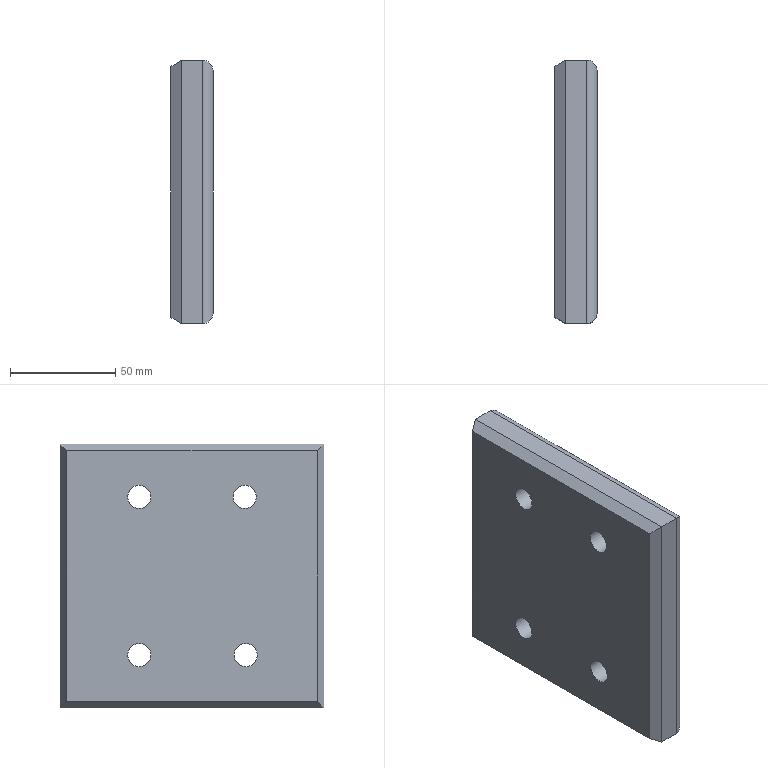Part | NX | features solid 2 | 1 solid | 30 faces | box 20 x 125 x 125 mm | volume 291132 mm3 | plane 14 | cylinder 12 | torus 4 | commonest cylinder face diameters 10 x4 11 x4 17.5 x4
STEP:
#1=CARTESIAN_POINT('',(1235.,-267.5,130.));
#2=VERTEX_POINT('',#1);
#3=CARTESIAN_POINT('',(1225.,-267.5,130.));
#4=VERTEX_POINT('',#3);
#5=CARTESIAN_POINT('',(1240.,-267.5,130.));
#6=DIRECTION('',(-1.,0.,0.));
#7=VECTOR('',#6,1000.);
#8=LINE('',#5,#7);
#9=EDGE_CURVE('',#2,#4,#8,.T.);
#10=ORIENTED_EDGE('',*,*,#9,.F.);
#11=CARTESIAN_POINT('',(1235.,-392.5,130.));
#12=VERTEX_POINT('',#11);
#13=CARTESIAN_POINT('',(1235.,-392.5,130.));
#14=DIRECTION('',(0.,-1.,0.));
#15=VECTOR('',#14,1000.);
#16=LINE('',#13,#15);
#17=EDGE_CURVE('',#12,#2,#16,.F.);
#18=ORIENTED_EDGE('',*,*,#17,.F.);
#19=CARTESIAN_POINT('',(1225.,-392.5,130.));
#20=VERTEX_POINT('',#19);
#21=CARTESIAN_POINT('',(1225.,-392.5,130.));
#22=CARTESIAN_POINT('',(1228.333,-392.5,130.));
#23=CARTESIAN_POINT('',(1231.667,-392.5,130.));
#24=CARTESIAN_POINT('',(1235.,-392.5,130.));
#25=B_SPLINE_CURVE_WITH_KNOTS('',3,(#21,#22,#23,#24),.UNSPECIFIED.,.F.,.F.,(4,4),(0.25,0.75),.UNSPECIFIED.);
#26=EDGE_CURVE('',#12,#20,#25,.F.);
#27=ORIENTED_EDGE('',*,*,#26,.T.);
#28=CARTESIAN_POINT('',(1225.,-392.5,130.));
#29=DIRECTION('',(0.,-1.,0.));
#30=VECTOR('',#29,1000.);
#31=LINE('',#28,#30);
#32=EDGE_CURVE('',#4,#20,#31,.T.);
#33=ORIENTED_EDGE('',*,*,#32,.F.);
#34=EDGE_LOOP('',(#10,#18,#27,#33));
#35=FACE_BOUND('',#34,.T.);
#36=CARTESIAN_POINT('',(1240.,-392.5,130.));
#37=DIRECTION('',(0.,0.,-1.));
#38=DIRECTION('',(1.,0.,0.));
#39=AXIS2_PLACEMENT_3D('',#36,#37,#38);
#40=PLANE('',#39);
#41=ADVANCED_FACE('',(#35),#40,.T.);
#42=ORIENTED_EDGE('',*,*,#26,.F.);
#43=CARTESIAN_POINT('',(1235.,-392.5,255.));
#44=VERTEX_POINT('',#43);
#45=CARTESIAN_POINT('',(1235.,-392.5,200.));
#46=DIRECTION('',(0.,0.,1.));
#47=VECTOR('',#46,1000.);
#48=LINE('',#45,#47);
#49=EDGE_CURVE('',#44,#12,#48,.F.);
#50=ORIENTED_EDGE('',*,*,#49,.F.);
#51=CARTESIAN_POINT('',(1225.,-392.5,255.));
#52=VERTEX_POINT('',#51);
#53=CARTESIAN_POINT('',(1240.,-392.5,255.));
#54=DIRECTION('',(-1.,0.,0.));
#55=VECTOR('',#54,1000.);
#56=LINE('',#53,#55);
#57=EDGE_CURVE('',#44,#52,#56,.T.);
#58=ORIENTED_EDGE('',*,*,#57,.T.);
#59=CARTESIAN_POINT('',(1225.,-392.5,255.));
#60=DIRECTION('',(0.,0.,1.));
#61=VECTOR('',#60,1000.);
#62=LINE('',#59,#61);
#63=EDGE_CURVE('',#20,#52,#62,.T.);
#64=ORIENTED_EDGE('',*,*,#63,.F.);
#65=EDGE_LOOP('',(#42,#50,#58,#64));
#66=FACE_BOUND('',#65,.T.);
#67=CARTESIAN_POINT('',(1240.,-392.5,200.));
#68=DIRECTION('',(0.,-1.,0.));
#69=DIRECTION('',(0.,0.,-1.));
#70=AXIS2_PLACEMENT_3D('',#67,#68,#69);
#71=PLANE('',#70);
#72=ADVANCED_FACE('',(#66),#71,.T.);
#73=ORIENTED_EDGE('',*,*,#57,.F.);
#74=CARTESIAN_POINT('',(1235.,-267.5,255.));
#75=VERTEX_POINT('',#74);
#76=CARTESIAN_POINT('',(1235.,-392.5,255.));
#77=DIRECTION('',(0.,-1.,0.));
#78=VECTOR('',#77,1000.);
#79=LINE('',#76,#78);
#80=EDGE_CURVE('',#75,#44,#79,.T.);
#81=ORIENTED_EDGE('',*,*,#80,.F.);
#82=CARTESIAN_POINT('',(1225.,-267.5,255.));
#83=VERTEX_POINT('',#82);
#84=CARTESIAN_POINT('',(1240.,-267.5,255.));
#85=DIRECTION('',(-1.,0.,0.));
#86=VECTOR('',#85,1000.);
#87=LINE('',#84,#86);
#88=EDGE_CURVE('',#75,#83,#87,.T.);
#89=ORIENTED_EDGE('',*,*,#88,.T.);
#90=CARTESIAN_POINT('',(1225.,-392.5,255.));
#91=DIRECTION('',(0.,1.,0.));
#92=VECTOR('',#91,1000.);
#93=LINE('',#90,#92);
#94=EDGE_CURVE('',#52,#83,#93,.T.);
#95=ORIENTED_EDGE('',*,*,#94,.F.);
#96=EDGE_LOOP('',(#73,#81,#89,#95));
#97=FACE_BOUND('',#96,.T.);
#98=CARTESIAN_POINT('',(1240.,-392.5,255.));
#99=DIRECTION('',(0.,0.,-1.));
#100=DIRECTION('',(1.,0.,0.));
#101=AXIS2_PLACEMENT_3D('',#98,#99,#100);
#102=PLANE('',#101);
#103=ADVANCED_FACE('',(#97),#102,.F.);
#104=ORIENTED_EDGE('',*,*,#88,.F.);
#105=CARTESIAN_POINT('',(1235.,-267.5,255.));
#106=DIRECTION('',(0.,0.,1.));
#107=VECTOR('',#106,1000.);
#108=LINE('',#105,#107);
#109=EDGE_CURVE('',#2,#75,#108,.T.);
#110=ORIENTED_EDGE('',*,*,#109,.F.);
#111=ORIENTED_EDGE('',*,*,#9,.T.);
#112=CARTESIAN_POINT('',(1225.,-267.5,200.));
#113=DIRECTION('',(0.,0.,-1.));
#114=VECTOR('',#113,1000.);
#115=LINE('',#112,#114);
#116=EDGE_CURVE('',#83,#4,#115,.T.);
#117=ORIENTED_EDGE('',*,*,#116,.F.);
#118=EDGE_LOOP('',(#104,#110,#111,#117));
#119=FACE_BOUND('',#118,.T.);
#120=CARTESIAN_POINT('',(1240.,-267.5,200.));
#121=DIRECTION('',(0.,-1.,0.));
#122=DIRECTION('',(0.,0.,-1.));
#123=AXIS2_PLACEMENT_3D('',#120,#121,#122);
#124=PLANE('',#123);
#125=ADVANCED_FACE('',(#119),#124,.F.);
#126=CARTESIAN_POINT('',(1240.,-355.,218.25));
#127=VERTEX_POINT('',#126);
#128=CARTESIAN_POINT('',(1240.,-355.,230.));
#129=DIRECTION('',(1.,0.,0.));
#130=DIRECTION('',(0.,0.,-1.));
#131=AXIS2_PLACEMENT_3D('',#128,#129,#130);
#132=CIRCLE('',#131,11.75);
#133=EDGE_CURVE('',#127,#127,#132,.T.);
#134=ORIENTED_EDGE('',*,*,#133,.F.);
#135=EDGE_LOOP('',(#134));
#136=FACE_BOUND('',#135,.T.);
#137=CARTESIAN_POINT('',(1240.,-305.,218.25));
#138=VERTEX_POINT('',#137);
#139=CARTESIAN_POINT('',(1240.,-305.,230.));
#140=DIRECTION('',(1.,0.,0.));
#141=DIRECTION('',(0.,0.,-1.));
#142=AXIS2_PLACEMENT_3D('',#139,#140,#141);
#143=CIRCLE('',#142,11.75);
#144=EDGE_CURVE('',#138,#138,#143,.T.);
#145=ORIENTED_EDGE('',*,*,#144,.F.);
#146=EDGE_LOOP('',(#145));
#147=FACE_BOUND('',#146,.T.);
#148=CARTESIAN_POINT('',(1240.,-305.,143.25));
#149=VERTEX_POINT('',#148);
#150=CARTESIAN_POINT('',(1240.,-305.,155.));
#151=DIRECTION('',(1.,0.,0.));
#152=DIRECTION('',(0.,0.,-1.));
#153=AXIS2_PLACEMENT_3D('',#150,#151,#152);
#154=CIRCLE('',#153,11.75);
#155=EDGE_CURVE('',#149,#149,#154,.T.);
#156=ORIENTED_EDGE('',*,*,#155,.F.);
#157=EDGE_LOOP('',(#156));
#158=FACE_BOUND('',#157,.T.);
#159=CARTESIAN_POINT('',(1240.,-355.5,143.25));
#160=VERTEX_POINT('',#159);
#161=CARTESIAN_POINT('',(1240.,-355.5,155.));
#162=DIRECTION('',(1.,0.,0.));
#163=DIRECTION('',(0.,0.,-1.));
#164=AXIS2_PLACEMENT_3D('',#161,#162,#163);
#165=CIRCLE('',#164,11.75);
#166=EDGE_CURVE('',#160,#160,#165,.T.);
#167=ORIENTED_EDGE('',*,*,#166,.F.);
#168=EDGE_LOOP('',(#167));
#169=FACE_BOUND('',#168,.T.);
#170=CARTESIAN_POINT('',(1240.,-387.5,135.));
#171=VERTEX_POINT('',#170);
#172=CARTESIAN_POINT('',(1240.,-387.5,250.));
#173=VERTEX_POINT('',#172);
#174=CARTESIAN_POINT('',(1240.,-387.5,200.));
#175=DIRECTION('',(0.,0.,-1.));
#176=VECTOR('',#175,1000.);
#177=LINE('',#174,#176);
#178=EDGE_CURVE('',#171,#173,#177,.F.);
#179=ORIENTED_EDGE('',*,*,#178,.F.);
#180=CARTESIAN_POINT('',(1240.,-272.5,135.));
#181=VERTEX_POINT('',#180);
#182=CARTESIAN_POINT('',(1240.,-392.5,135.));
#183=DIRECTION('',(0.,1.,0.));
#184=VECTOR('',#183,1000.);
#185=LINE('',#182,#184);
#186=EDGE_CURVE('',#181,#171,#185,.F.);
#187=ORIENTED_EDGE('',*,*,#186,.F.);
#188=CARTESIAN_POINT('',(1240.,-272.5,250.));
#189=VERTEX_POINT('',#188);
#190=CARTESIAN_POINT('',(1240.,-272.5,130.));
#191=DIRECTION('',(0.,0.,-1.));
#192=VECTOR('',#191,1000.);
#193=LINE('',#190,#192);
#194=EDGE_CURVE('',#189,#181,#193,.T.);
#195=ORIENTED_EDGE('',*,*,#194,.F.);
#196=CARTESIAN_POINT('',(1240.,-267.5,250.));
#197=DIRECTION('',(0.,1.,0.));
#198=VECTOR('',#197,1000.);
#199=LINE('',#196,#198);
#200=EDGE_CURVE('',#173,#189,#199,.T.);
#201=ORIENTED_EDGE('',*,*,#200,.F.);
#202=EDGE_LOOP('',(#179,#187,#195,#201));
#203=FACE_BOUND('',#202,.T.);
#204=CARTESIAN_POINT('',(1240.,-392.5,200.));
#205=DIRECTION('',(-1.,0.,0.));
#206=DIRECTION('',(0.,0.,-1.));
#207=AXIS2_PLACEMENT_3D('',#204,#205,#206);
#208=PLANE('',#207);
#209=ADVANCED_FACE('',(#136,#147,#158,#169,#203),#208,.F.);
#210=CARTESIAN_POINT('',(1220.,-389.5,133.));
#211=VERTEX_POINT('',#210);
#212=CARTESIAN_POINT('',(1220.,-270.5,133.));
#213=VERTEX_POINT('',#212);
#214=CARTESIAN_POINT('',(1220.,-267.5,133.));
#215=DIRECTION('',(0.,-1.,0.));
#216=VECTOR('',#215,1000.);
#217=LINE('',#214,#216);
#218=EDGE_CURVE('',#211,#213,#217,.F.);
#219=ORIENTED_EDGE('',*,*,#218,.F.);
#220=CARTESIAN_POINT('',(1220.,-389.5,252.));
#221=VERTEX_POINT('',#220);
#222=CARTESIAN_POINT('',(1220.,-389.5,130.));
#223=DIRECTION('',(0.,0.,1.));
#224=VECTOR('',#223,1000.);
#225=LINE('',#222,#224);
#226=EDGE_CURVE('',#221,#211,#225,.F.);
#227=ORIENTED_EDGE('',*,*,#226,.F.);
#228=CARTESIAN_POINT('',(1220.,-270.5,252.));
#229=VERTEX_POINT('',#228);
#230=CARTESIAN_POINT('',(1220.,-392.5,252.));
#231=DIRECTION('',(0.,1.,0.));
#232=VECTOR('',#231,1000.);
#233=LINE('',#230,#232);
#234=EDGE_CURVE('',#229,#221,#233,.F.);
#235=ORIENTED_EDGE('',*,*,#234,.F.);
#236=CARTESIAN_POINT('',(1220.,-270.5,200.));
#237=DIRECTION('',(0.,0.,-1.));
#238=VECTOR('',#237,1000.);
#239=LINE('',#236,#238);
#240=EDGE_CURVE('',#213,#229,#239,.F.);
#241=ORIENTED_EDGE('',*,*,#240,.F.);
#242=EDGE_LOOP('',(#219,#227,#235,#241));
#243=FACE_BOUND('',#242,.T.);
#244=CARTESIAN_POINT('',(1220.,-305.,224.5));
#245=VERTEX_POINT('',#244);
#246=CARTESIAN_POINT('',(1220.,-305.,230.));
#247=DIRECTION('',(1.,0.,0.));
#248=DIRECTION('',(0.,0.,-1.));
#249=AXIS2_PLACEMENT_3D('',#246,#247,#248);
#250=CIRCLE('',#249,5.5);
#251=EDGE_CURVE('',#245,#245,#250,.F.);
#252=ORIENTED_EDGE('',*,*,#251,.F.);
#253=EDGE_LOOP('',(#252));
#254=FACE_BOUND('',#253,.T.);
#255=CARTESIAN_POINT('',(1220.,-355.,224.5));
#256=VERTEX_POINT('',#255);
#257=CARTESIAN_POINT('',(1220.,-355.,230.));
#258=DIRECTION('',(1.,0.,0.));
#259=DIRECTION('',(0.,0.,-1.));
#260=AXIS2_PLACEMENT_3D('',#257,#258,#259);
#261=CIRCLE('',#260,5.5);
#262=EDGE_CURVE('',#256,#256,#261,.F.);
#263=ORIENTED_EDGE('',*,*,#262,.F.);
#264=EDGE_LOOP('',(#263));
#265=FACE_BOUND('',#264,.T.);
#266=CARTESIAN_POINT('',(1220.,-305.,149.5));
#267=VERTEX_POINT('',#266);
#268=CARTESIAN_POINT('',(1220.,-305.,155.));
#269=DIRECTION('',(1.,0.,0.));
#270=DIRECTION('',(0.,0.,-1.));
#271=AXIS2_PLACEMENT_3D('',#268,#269,#270);
#272=CIRCLE('',#271,5.5);
#273=EDGE_CURVE('',#267,#267,#272,.F.);
#274=ORIENTED_EDGE('',*,*,#273,.F.);
#275=EDGE_LOOP('',(#274));
#276=FACE_BOUND('',#275,.T.);
#277=CARTESIAN_POINT('',(1220.,-355.5,149.5));
#278=VERTEX_POINT('',#277);
#279=CARTESIAN_POINT('',(1220.,-355.5,155.));
#280=DIRECTION('',(1.,0.,0.));
#281=DIRECTION('',(0.,0.,-1.));
#282=AXIS2_PLACEMENT_3D('',#279,#280,#281);
#283=CIRCLE('',#282,5.5);
#284=EDGE_CURVE('',#278,#278,#283,.F.);
#285=ORIENTED_EDGE('',*,*,#284,.F.);
#286=EDGE_LOOP('',(#285));
#287=FACE_BOUND('',#286,.T.);
#288=CARTESIAN_POINT('',(1220.,-392.5,200.));
#289=DIRECTION('',(-1.,0.,0.));
#290=DIRECTION('',(0.,0.,-1.));
#291=AXIS2_PLACEMENT_3D('',#288,#289,#290);
#292=PLANE('',#291);
#293=ADVANCED_FACE('',(#243,#254,#265,#276,#287),#292,.T.);
#294=CARTESIAN_POINT('',(1228.,-355.5,149.5));
#295=VERTEX_POINT('',#294);
#296=CARTESIAN_POINT('',(1228.,-355.5,155.));
#297=DIRECTION('',(1.,0.,0.));
#298=DIRECTION('',(0.,0.,-1.));
#299=AXIS2_PLACEMENT_3D('',#296,#297,#298);
#300=CIRCLE('',#299,5.5);
#301=EDGE_CURVE('',#295,#295,#300,.T.);
#302=ORIENTED_EDGE('',*,*,#301,.T.);
#303=EDGE_LOOP('',(#302));
#304=FACE_BOUND('',#303,.T.);
#305=ORIENTED_EDGE('',*,*,#284,.T.);
#306=EDGE_LOOP('',(#305));
#307=FACE_BOUND('',#306,.T.);
#308=CARTESIAN_POINT('',(1190.,-355.5,155.));
#309=DIRECTION('',(-1.,0.,0.));
#310=DIRECTION('',(0.,0.,-1.));
#311=AXIS2_PLACEMENT_3D('',#308,#309,#310);
#312=CYLINDRICAL_SURFACE('',#311,5.5);
#313=ADVANCED_FACE('',(#304,#307),#312,.F.);
#314=ORIENTED_EDGE('',*,*,#301,.F.);
#315=EDGE_LOOP('',(#314));
#316=FACE_BOUND('',#315,.T.);
#317=CARTESIAN_POINT('',(1228.,-355.5,146.25));
#318=VERTEX_POINT('',#317);
#319=CARTESIAN_POINT('',(1228.,-355.5,155.));
#320=DIRECTION('',(1.,0.,0.));
#321=DIRECTION('',(0.,0.,-1.));
#322=AXIS2_PLACEMENT_3D('',#319,#320,#321);
#323=CIRCLE('',#322,8.75);
#324=EDGE_CURVE('',#318,#318,#323,.T.);
#325=ORIENTED_EDGE('',*,*,#324,.T.);
#326=EDGE_LOOP('',(#325));
#327=FACE_BOUND('',#326,.T.);
#328=CARTESIAN_POINT('',(1228.,-355.5,155.));
#329=DIRECTION('',(-1.,0.,0.));
#330=DIRECTION('',(0.,0.,-1.));
#331=AXIS2_PLACEMENT_3D('',#328,#329,#330);
#332=PLANE('',#331);
#333=ADVANCED_FACE('',(#316,#327),#332,.F.);
#334=CARTESIAN_POINT('',(1237.,-355.5,146.25));
#335=VERTEX_POINT('',#334);
#336=CARTESIAN_POINT('',(1237.,-355.5,155.));
#337=DIRECTION('',(1.,0.,0.));
#338=DIRECTION('',(0.,0.,-1.));
#339=AXIS2_PLACEMENT_3D('',#336,#337,#338);
#340=CIRCLE('',#339,8.75);
#341=EDGE_CURVE('',#335,#335,#340,.F.);
#342=ORIENTED_EDGE('',*,*,#341,.F.);
#343=EDGE_LOOP('',(#342));
#344=FACE_BOUND('',#343,.T.);
#345=ORIENTED_EDGE('',*,*,#324,.F.);
#346=EDGE_LOOP('',(#345));
#347=FACE_BOUND('',#346,.T.);
#348=CARTESIAN_POINT('',(1240.,-355.5,155.));
#349=DIRECTION('',(-1.,0.,0.));
#350=DIRECTION('',(0.,0.,-1.));
#351=AXIS2_PLACEMENT_3D('',#348,#349,#350);
#352=CYLINDRICAL_SURFACE('',#351,8.75);
#353=ADVANCED_FACE('',(#344,#347),#352,.F.);
#354=CARTESIAN_POINT('',(1228.,-305.,149.5));
#355=VERTEX_POINT('',#354);
#356=CARTESIAN_POINT('',(1228.,-305.,155.));
#357=DIRECTION('',(1.,0.,0.));
#358=DIRECTION('',(0.,0.,-1.));
#359=AXIS2_PLACEMENT_3D('',#356,#357,#358);
#360=CIRCLE('',#359,5.5);
#361=EDGE_CURVE('',#355,#355,#360,.T.);
#362=ORIENTED_EDGE('',*,*,#361,.T.);
#363=EDGE_LOOP('',(#362));
#364=FACE_BOUND('',#363,.T.);
#365=ORIENTED_EDGE('',*,*,#273,.T.);
#366=EDGE_LOOP('',(#365));
#367=FACE_BOUND('',#366,.T.);
#368=CARTESIAN_POINT('',(1190.,-305.,155.));
#369=DIRECTION('',(-1.,0.,0.));
#370=DIRECTION('',(0.,0.,-1.));
#371=AXIS2_PLACEMENT_3D('',#368,#369,#370);
#372=CYLINDRICAL_SURFACE('',#371,5.5);
#373=ADVANCED_FACE('',(#364,#367),#372,.F.);
#374=ORIENTED_EDGE('',*,*,#361,.F.);
#375=EDGE_LOOP('',(#374));
#376=FACE_BOUND('',#375,.T.);
#377=CARTESIAN_POINT('',(1228.,-305.,146.25));
#378=VERTEX_POINT('',#377);
#379=CARTESIAN_POINT('',(1228.,-305.,155.));
#380=DIRECTION('',(1.,0.,0.));
#381=DIRECTION('',(0.,0.,-1.));
#382=AXIS2_PLACEMENT_3D('',#379,#380,#381);
#383=CIRCLE('',#382,8.75);
#384=EDGE_CURVE('',#378,#378,#383,.T.);
#385=ORIENTED_EDGE('',*,*,#384,.T.);
#386=EDGE_LOOP('',(#385));
#387=FACE_BOUND('',#386,.T.);
#388=CARTESIAN_POINT('',(1228.,-305.,155.));
#389=DIRECTION('',(-1.,0.,0.));
#390=DIRECTION('',(0.,0.,-1.));
#391=AXIS2_PLACEMENT_3D('',#388,#389,#390);
#392=PLANE('',#391);
#393=ADVANCED_FACE('',(#376,#387),#392,.F.);
#394=CARTESIAN_POINT('',(1237.,-305.,146.25));
#395=VERTEX_POINT('',#394);
#396=CARTESIAN_POINT('',(1237.,-305.,155.));
#397=DIRECTION('',(1.,0.,0.));
#398=DIRECTION('',(0.,0.,-1.));
#399=AXIS2_PLACEMENT_3D('',#396,#397,#398);
#400=CIRCLE('',#399,8.75);
#401=EDGE_CURVE('',#395,#395,#400,.F.);
#402=ORIENTED_EDGE('',*,*,#401,.F.);
#403=EDGE_LOOP('',(#402));
#404=FACE_BOUND('',#403,.T.);
#405=ORIENTED_EDGE('',*,*,#384,.F.);
#406=EDGE_LOOP('',(#405));
#407=FACE_BOUND('',#406,.T.);
#408=CARTESIAN_POINT('',(1240.,-305.,155.));
#409=DIRECTION('',(-1.,0.,0.));
#410=DIRECTION('',(0.,0.,-1.));
#411=AXIS2_PLACEMENT_3D('',#408,#409,#410);
#412=CYLINDRICAL_SURFACE('',#411,8.75);
#413=ADVANCED_FACE('',(#404,#407),#412,.F.);
#414=CARTESIAN_POINT('',(1228.,-355.,224.5));
#415=VERTEX_POINT('',#414);
#416=CARTESIAN_POINT('',(1228.,-355.,230.));
#417=DIRECTION('',(1.,0.,0.));
#418=DIRECTION('',(0.,0.,-1.));
#419=AXIS2_PLACEMENT_3D('',#416,#417,#418);
#420=CIRCLE('',#419,5.5);
#421=EDGE_CURVE('',#415,#415,#420,.T.);
#422=ORIENTED_EDGE('',*,*,#421,.T.);
#423=EDGE_LOOP('',(#422));
#424=FACE_BOUND('',#423,.T.);
#425=ORIENTED_EDGE('',*,*,#262,.T.);
#426=EDGE_LOOP('',(#425));
#427=FACE_BOUND('',#426,.T.);
#428=CARTESIAN_POINT('',(1190.,-355.,230.));
#429=DIRECTION('',(-1.,0.,0.));
#430=DIRECTION('',(0.,0.,-1.));
#431=AXIS2_PLACEMENT_3D('',#428,#429,#430);
#432=CYLINDRICAL_SURFACE('',#431,5.5);
#433=ADVANCED_FACE('',(#424,#427),#432,.F.);
#434=ORIENTED_EDGE('',*,*,#421,.F.);
#435=EDGE_LOOP('',(#434));
#436=FACE_BOUND('',#435,.T.);
#437=CARTESIAN_POINT('',(1228.,-355.,221.25));
#438=VERTEX_POINT('',#437);
#439=CARTESIAN_POINT('',(1228.,-355.,230.));
#440=DIRECTION('',(1.,0.,0.));
#441=DIRECTION('',(0.,0.,-1.));
#442=AXIS2_PLACEMENT_3D('',#439,#440,#441);
#443=CIRCLE('',#442,8.75);
#444=EDGE_CURVE('',#438,#438,#443,.T.);
#445=ORIENTED_EDGE('',*,*,#444,.T.);
#446=EDGE_LOOP('',(#445));
#447=FACE_BOUND('',#446,.T.);
#448=CARTESIAN_POINT('',(1228.,-355.,230.));
#449=DIRECTION('',(-1.,0.,0.));
#450=DIRECTION('',(0.,0.,-1.));
#451=AXIS2_PLACEMENT_3D('',#448,#449,#450);
#452=PLANE('',#451);
#453=ADVANCED_FACE('',(#436,#447),#452,.F.);
#454=CARTESIAN_POINT('',(1237.,-355.,221.25));
#455=VERTEX_POINT('',#454);
#456=CARTESIAN_POINT('',(1237.,-355.,230.));
#457=DIRECTION('',(1.,0.,0.));
#458=DIRECTION('',(0.,0.,-1.));
#459=AXIS2_PLACEMENT_3D('',#456,#457,#458);
#460=CIRCLE('',#459,8.75);
#461=EDGE_CURVE('',#455,#455,#460,.F.);
#462=ORIENTED_EDGE('',*,*,#461,.F.);
#463=EDGE_LOOP('',(#462));
#464=FACE_BOUND('',#463,.T.);
#465=ORIENTED_EDGE('',*,*,#444,.F.);
#466=EDGE_LOOP('',(#465));
#467=FACE_BOUND('',#466,.T.);
#468=CARTESIAN_POINT('',(1240.,-355.,230.));
#469=DIRECTION('',(-1.,0.,0.));
#470=DIRECTION('',(0.,0.,-1.));
#471=AXIS2_PLACEMENT_3D('',#468,#469,#470);
#472=CYLINDRICAL_SURFACE('',#471,8.75);
#473=ADVANCED_FACE('',(#464,#467),#472,.F.);
#474=CARTESIAN_POINT('',(1228.,-305.,224.5));
#475=VERTEX_POINT('',#474);
#476=CARTESIAN_POINT('',(1228.,-305.,230.));
#477=DIRECTION('',(1.,0.,0.));
#478=DIRECTION('',(0.,0.,-1.));
#479=AXIS2_PLACEMENT_3D('',#476,#477,#478);
#480=CIRCLE('',#479,5.5);
#481=EDGE_CURVE('',#475,#475,#480,.T.);
#482=ORIENTED_EDGE('',*,*,#481,.T.);
#483=EDGE_LOOP('',(#482));
#484=FACE_BOUND('',#483,.T.);
#485=ORIENTED_EDGE('',*,*,#251,.T.);
#486=EDGE_LOOP('',(#485));
#487=FACE_BOUND('',#486,.T.);
#488=CARTESIAN_POINT('',(1190.,-305.,230.));
#489=DIRECTION('',(-1.,0.,0.));
#490=DIRECTION('',(0.,0.,-1.));
#491=AXIS2_PLACEMENT_3D('',#488,#489,#490);
#492=CYLINDRICAL_SURFACE('',#491,5.5);
#493=ADVANCED_FACE('',(#484,#487),#492,.F.);
#494=ORIENTED_EDGE('',*,*,#481,.F.);
#495=EDGE_LOOP('',(#494));
#496=FACE_BOUND('',#495,.T.);
#497=CARTESIAN_POINT('',(1228.,-305.,221.25));
#498=VERTEX_POINT('',#497);
#499=CARTESIAN_POINT('',(1228.,-305.,230.));
#500=DIRECTION('',(1.,0.,0.));
#501=DIRECTION('',(0.,0.,-1.));
#502=AXIS2_PLACEMENT_3D('',#499,#500,#501);
#503=CIRCLE('',#502,8.75);
#504=EDGE_CURVE('',#498,#498,#503,.T.);
#505=ORIENTED_EDGE('',*,*,#504,.T.);
#506=EDGE_LOOP('',(#505));
#507=FACE_BOUND('',#506,.T.);
#508=CARTESIAN_POINT('',(1228.,-305.,230.));
#509=DIRECTION('',(-1.,0.,0.));
#510=DIRECTION('',(0.,0.,-1.));
#511=AXIS2_PLACEMENT_3D('',#508,#509,#510);
#512=PLANE('',#511);
#513=ADVANCED_FACE('',(#496,#507),#512,.F.);
#514=CARTESIAN_POINT('',(1237.,-305.,221.25));
#515=VERTEX_POINT('',#514);
#516=CARTESIAN_POINT('',(1237.,-305.,230.));
#517=DIRECTION('',(1.,0.,0.));
#518=DIRECTION('',(0.,0.,-1.));
#519=AXIS2_PLACEMENT_3D('',#516,#517,#518);
#520=CIRCLE('',#519,8.75);
#521=EDGE_CURVE('',#515,#515,#520,.F.);
#522=ORIENTED_EDGE('',*,*,#521,.F.);
#523=EDGE_LOOP('',(#522));
#524=FACE_BOUND('',#523,.T.);
#525=ORIENTED_EDGE('',*,*,#504,.F.);
#526=EDGE_LOOP('',(#525));
#527=FACE_BOUND('',#526,.T.);
#528=CARTESIAN_POINT('',(1240.,-305.,230.));
#529=DIRECTION('',(-1.,0.,0.));
#530=DIRECTION('',(0.,0.,-1.));
#531=AXIS2_PLACEMENT_3D('',#528,#529,#530);
#532=CYLINDRICAL_SURFACE('',#531,8.75);
#533=ADVANCED_FACE('',(#524,#527),#532,.F.);
#534=CARTESIAN_POINT('',(1235.,-272.5,135.));
#535=DIRECTION('',(0.,0.7071,0.7071));
#536=DIRECTION('',(0.,-0.7071,0.7071));
#537=AXIS2_PLACEMENT_3D('',#534,#535,#536);
#538=ELLIPSE('',#537,7.071,5.);
#539=EDGE_CURVE('',#2,#181,#538,.F.);
#540=ORIENTED_EDGE('',*,*,#539,.T.);
#541=ORIENTED_EDGE('',*,*,#186,.T.);
#542=CARTESIAN_POINT('',(1235.,-387.5,135.));
#543=DIRECTION('',(0.,0.7071,-0.7071));
#544=DIRECTION('',(0.,0.7071,0.7071));
#545=AXIS2_PLACEMENT_3D('',#542,#543,#544);
#546=ELLIPSE('',#545,7.071,5.);
#547=EDGE_CURVE('',#171,#12,#546,.T.);
#548=ORIENTED_EDGE('',*,*,#547,.T.);
#549=ORIENTED_EDGE('',*,*,#17,.T.);
#550=EDGE_LOOP('',(#540,#541,#548,#549));
#551=FACE_BOUND('',#550,.T.);
#552=CARTESIAN_POINT('',(1235.,-392.5,135.));
#553=DIRECTION('',(0.,-1.,0.));
#554=DIRECTION('',(0.,0.,-1.));
#555=AXIS2_PLACEMENT_3D('',#552,#553,#554);
#556=CYLINDRICAL_SURFACE('',#555,5.);
#557=ADVANCED_FACE('',(#551),#556,.T.);
#558=ORIENTED_EDGE('',*,*,#547,.F.);
#559=ORIENTED_EDGE('',*,*,#178,.T.);
#560=CARTESIAN_POINT('',(1235.,-387.5,250.));
#561=DIRECTION('',(0.,-0.7071,-0.7071));
#562=DIRECTION('',(0.,-0.7071,0.7071));
#563=AXIS2_PLACEMENT_3D('',#560,#561,#562);
#564=ELLIPSE('',#563,7.071,5.);
#565=EDGE_CURVE('',#173,#44,#564,.T.);
#566=ORIENTED_EDGE('',*,*,#565,.T.);
#567=ORIENTED_EDGE('',*,*,#49,.T.);
#568=EDGE_LOOP('',(#558,#559,#566,#567));
#569=FACE_BOUND('',#568,.T.);
#570=CARTESIAN_POINT('',(1235.,-387.5,200.));
#571=DIRECTION('',(0.,0.,1.));
#572=DIRECTION('',(-1.,0.,0.));
#573=AXIS2_PLACEMENT_3D('',#570,#571,#572);
#574=CYLINDRICAL_SURFACE('',#573,5.);
#575=ADVANCED_FACE('',(#569),#574,.T.);
#576=ORIENTED_EDGE('',*,*,#539,.F.);
#577=ORIENTED_EDGE('',*,*,#109,.T.);
#578=CARTESIAN_POINT('',(1235.,-272.5,250.));
#579=DIRECTION('',(0.,-0.7071,0.7071));
#580=DIRECTION('',(0.,-0.7071,-0.7071));
#581=AXIS2_PLACEMENT_3D('',#578,#579,#580);
#582=ELLIPSE('',#581,7.071,5.);
#583=EDGE_CURVE('',#75,#189,#582,.F.);
#584=ORIENTED_EDGE('',*,*,#583,.T.);
#585=ORIENTED_EDGE('',*,*,#194,.T.);
#586=EDGE_LOOP('',(#576,#577,#584,#585));
#587=FACE_BOUND('',#586,.T.);
#588=CARTESIAN_POINT('',(1235.,-272.5,200.));
#589=DIRECTION('',(0.,0.,-1.));
#590=DIRECTION('',(1.,0.,0.));
#591=AXIS2_PLACEMENT_3D('',#588,#589,#590);
#592=CYLINDRICAL_SURFACE('',#591,5.);
#593=ADVANCED_FACE('',(#587),#592,.T.);
#594=ORIENTED_EDGE('',*,*,#565,.F.);
#595=ORIENTED_EDGE('',*,*,#200,.T.);
#596=ORIENTED_EDGE('',*,*,#583,.F.);
#597=ORIENTED_EDGE('',*,*,#80,.T.);
#598=EDGE_LOOP('',(#594,#595,#596,#597));
#599=FACE_BOUND('',#598,.T.);
#600=CARTESIAN_POINT('',(1235.,-392.5,250.));
#601=DIRECTION('',(0.,1.,0.));
#602=DIRECTION('',(0.,0.,1.));
#603=AXIS2_PLACEMENT_3D('',#600,#601,#602);
#604=CYLINDRICAL_SURFACE('',#603,5.);
#605=ADVANCED_FACE('',(#599),#604,.T.);
#606=ORIENTED_EDGE('',*,*,#461,.T.);
#607=EDGE_LOOP('',(#606));
#608=FACE_BOUND('',#607,.T.);
#609=ORIENTED_EDGE('',*,*,#133,.T.);
#610=EDGE_LOOP('',(#609));
#611=FACE_BOUND('',#610,.T.);
#612=CARTESIAN_POINT('',(1237.,-355.,230.));
#613=DIRECTION('',(-1.,0.,0.));
#614=DIRECTION('',(0.,0.,-1.));
#615=AXIS2_PLACEMENT_3D('',#612,#613,#614);
#616=TOROIDAL_SURFACE('',#615,11.75,3.);
#617=ADVANCED_FACE('',(#608,#611),#616,.T.);
#618=ORIENTED_EDGE('',*,*,#521,.T.);
#619=EDGE_LOOP('',(#618));
#620=FACE_BOUND('',#619,.T.);
#621=ORIENTED_EDGE('',*,*,#144,.T.);
#622=EDGE_LOOP('',(#621));
#623=FACE_BOUND('',#622,.T.);
#624=CARTESIAN_POINT('',(1237.,-305.,230.));
#625=DIRECTION('',(-1.,0.,0.));
#626=DIRECTION('',(0.,0.,-1.));
#627=AXIS2_PLACEMENT_3D('',#624,#625,#626);
#628=TOROIDAL_SURFACE('',#627,11.75,3.);
#629=ADVANCED_FACE('',(#620,#623),#628,.T.);
#630=ORIENTED_EDGE('',*,*,#401,.T.);
#631=EDGE_LOOP('',(#630));
#632=FACE_BOUND('',#631,.T.);
#633=ORIENTED_EDGE('',*,*,#155,.T.);
#634=EDGE_LOOP('',(#633));
#635=FACE_BOUND('',#634,.T.);
#636=CARTESIAN_POINT('',(1237.,-305.,155.));
#637=DIRECTION('',(-1.,0.,0.));
#638=DIRECTION('',(0.,0.,-1.));
#639=AXIS2_PLACEMENT_3D('',#636,#637,#638);
#640=TOROIDAL_SURFACE('',#639,11.75,3.);
#641=ADVANCED_FACE('',(#632,#635),#640,.T.);
#642=ORIENTED_EDGE('',*,*,#341,.T.);
#643=EDGE_LOOP('',(#642));
#644=FACE_BOUND('',#643,.T.);
#645=ORIENTED_EDGE('',*,*,#166,.T.);
#646=EDGE_LOOP('',(#645));
#647=FACE_BOUND('',#646,.T.);
#648=CARTESIAN_POINT('',(1237.,-355.5,155.));
#649=DIRECTION('',(-1.,0.,0.));
#650=DIRECTION('',(0.,0.,-1.));
#651=AXIS2_PLACEMENT_3D('',#648,#649,#650);
#652=TOROIDAL_SURFACE('',#651,11.75,3.);
#653=ADVANCED_FACE('',(#644,#647),#652,.T.);
#654=CARTESIAN_POINT('',(1196.628,-375.477,147.023));
#655=DIRECTION('',(-0.7625,0.4575,0.4575));
#656=VECTOR('',#655,1000.);
#657=LINE('',#654,#656);
#658=EDGE_CURVE('',#211,#20,#657,.F.);
#659=ORIENTED_EDGE('',*,*,#658,.T.);
#660=ORIENTED_EDGE('',*,*,#63,.T.);
#661=CARTESIAN_POINT('',(1201.86,-378.616,241.116));
#662=DIRECTION('',(-0.7625,0.4575,-0.4575));
#663=VECTOR('',#662,1000.);
#664=LINE('',#661,#663);
#665=EDGE_CURVE('',#52,#221,#664,.T.);
#666=ORIENTED_EDGE('',*,*,#665,.T.);
#667=ORIENTED_EDGE('',*,*,#226,.T.);
#668=EDGE_LOOP('',(#659,#660,#666,#667));
#669=FACE_BOUND('',#668,.T.);
#670=CARTESIAN_POINT('',(1220.,-389.5,200.));
#671=DIRECTION('',(0.5145,0.8575,0.));
#672=DIRECTION('',(0.8575,-0.5145,0.));
#673=AXIS2_PLACEMENT_3D('',#670,#671,#672);
#674=PLANE('',#673);
#675=ADVANCED_FACE('',(#669),#674,.F.);
#676=ORIENTED_EDGE('',*,*,#665,.F.);
#677=ORIENTED_EDGE('',*,*,#94,.T.);
#678=CARTESIAN_POINT('',(1181.395,-293.663,228.837));
#679=DIRECTION('',(0.7625,0.4575,0.4575));
#680=VECTOR('',#679,1000.);
#681=LINE('',#678,#680);
#682=EDGE_CURVE('',#83,#229,#681,.F.);
#683=ORIENTED_EDGE('',*,*,#682,.T.);
#684=ORIENTED_EDGE('',*,*,#234,.T.);
#685=EDGE_LOOP('',(#676,#677,#683,#684));
#686=FACE_BOUND('',#685,.T.);
#687=CARTESIAN_POINT('',(1225.,-392.5,255.));
#688=DIRECTION('',(-0.5145,0.,0.8575));
#689=DIRECTION('',(-0.8575,0.,-0.5145));
#690=AXIS2_PLACEMENT_3D('',#687,#688,#689);
#691=PLANE('',#690);
#692=ADVANCED_FACE('',(#686),#691,.T.);
#693=ORIENTED_EDGE('',*,*,#658,.F.);
#694=ORIENTED_EDGE('',*,*,#218,.T.);
#695=CARTESIAN_POINT('',(1177.442,-296.035,158.535));
#696=DIRECTION('',(0.7625,0.4575,-0.4575));
#697=VECTOR('',#696,1000.);
#698=LINE('',#695,#697);
#699=EDGE_CURVE('',#213,#4,#698,.T.);
#700=ORIENTED_EDGE('',*,*,#699,.T.);
#701=ORIENTED_EDGE('',*,*,#32,.T.);
#702=EDGE_LOOP('',(#693,#694,#700,#701));
#703=FACE_BOUND('',#702,.T.);
#704=CARTESIAN_POINT('',(1220.,-392.5,133.));
#705=DIRECTION('',(0.5145,0.,0.8575));
#706=DIRECTION('',(-0.8575,0.,0.5145));
#707=AXIS2_PLACEMENT_3D('',#704,#705,#706);
#708=PLANE('',#707);
#709=ADVANCED_FACE('',(#703),#708,.F.);
#710=ORIENTED_EDGE('',*,*,#682,.F.);
#711=ORIENTED_EDGE('',*,*,#116,.T.);
#712=ORIENTED_EDGE('',*,*,#699,.F.);
#713=ORIENTED_EDGE('',*,*,#240,.T.);
#714=EDGE_LOOP('',(#710,#711,#712,#713));
#715=FACE_BOUND('',#714,.T.);
#716=CARTESIAN_POINT('',(1225.,-267.5,200.));
#717=DIRECTION('',(-0.5145,0.8575,0.));
#718=DIRECTION('',(0.8575,0.5145,0.));
#719=AXIS2_PLACEMENT_3D('',#716,#717,#718);
#720=PLANE('',#719);
#721=ADVANCED_FACE('',(#715),#720,.T.);
#722=CLOSED_SHELL('',(#41,#72,#103,#125,#209,#293,#313,#333,#353,#373,#393,#413,#433,#453,#473,#493,#513,#533,#557,#575,#593,#605,#617,#629,#641,#653,#675,#692,#709,#721));
#723=MANIFOLD_SOLID_BREP('',#722);
#724=(LENGTH_UNIT()NAMED_UNIT(*)SI_UNIT(.MILLI.,.METRE.));
#725=UNCERTAINTY_MEASURE_WITH_UNIT(LENGTH_MEASURE(0.0508),#724,'','');
#726=(NAMED_UNIT(*)PLANE_ANGLE_UNIT()SI_UNIT($,.RADIAN.));
#727=(NAMED_UNIT(*)SI_UNIT($,.STERADIAN.)SOLID_ANGLE_UNIT());
#728=(GEOMETRIC_REPRESENTATION_CONTEXT(3)GLOBAL_UNCERTAINTY_ASSIGNED_CONTEXT((#725))GLOBAL_UNIT_ASSIGNED_CONTEXT((#724,#726,#727))REPRESENTATION_CONTEXT('',''));
#729=ADVANCED_BREP_SHAPE_REPRESENTATION('',(#723),#728);